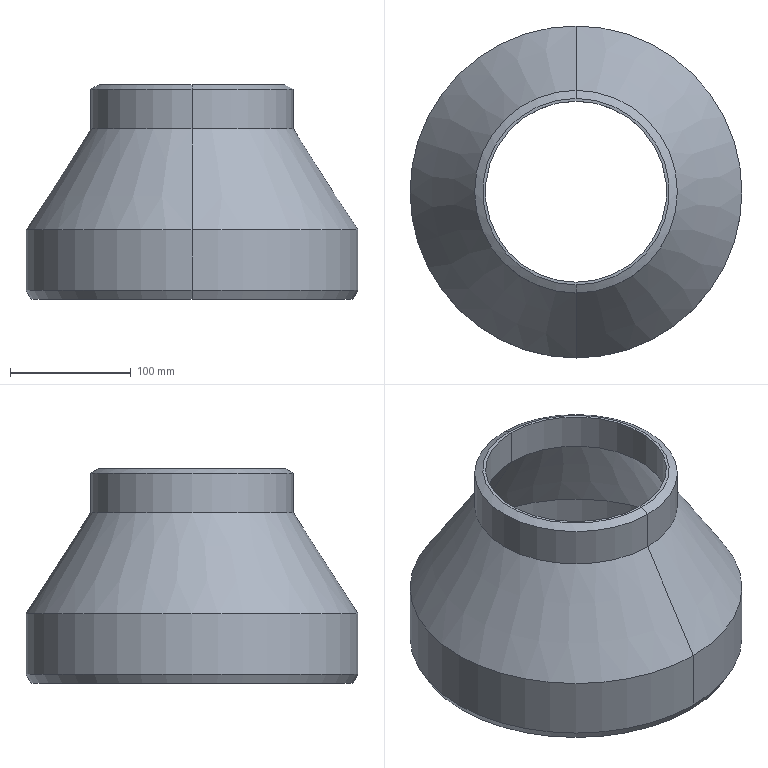Part | NX | features Resize Face 2, BREP 1 | 1 solid | 18 faces | box 275 x 275 x 178 mm | volume 1214659 mm3 | cone 8 | cylinder 8 | plane 2 | commonest cylinder face diameters 150 x2 168 x2 250 x2 275 x2
STEP:
#1=CARTESIAN_POINT('',(0.,-77.25,0.));
#2=VERTEX_POINT('',#1);
#3=CARTESIAN_POINT('',(0.,77.25,0.));
#4=VERTEX_POINT('',#3);
#5=CARTESIAN_POINT('',(0.,0.,0.));
#6=DIRECTION('',(0.,0.,1.));
#7=DIRECTION('',(0.,-1.,0.));
#8=AXIS2_PLACEMENT_3D('',#5,#6,#7);
#9=CIRCLE('',#8,77.25);
#10=EDGE_CURVE('',#2,#4,#9,.T.);
#11=ORIENTED_EDGE('',*,*,#10,.F.);
#12=CARTESIAN_POINT('',(0.,-84.,-3.897));
#13=VERTEX_POINT('',#12);
#14=CARTESIAN_POINT('',(0.,-79.5,-1.299));
#15=DIRECTION('',(0.,-0.866,-0.5));
#16=VECTOR('',#15,1000.);
#17=LINE('',#14,#16);
#18=EDGE_CURVE('',#2,#13,#17,.T.);
#19=ORIENTED_EDGE('',*,*,#18,.T.);
#20=CARTESIAN_POINT('',(0.,84.,-3.897));
#21=VERTEX_POINT('',#20);
#22=CARTESIAN_POINT('',(0.,0.,-3.897));
#23=DIRECTION('',(0.,0.,-1.));
#24=DIRECTION('',(0.,1.,0.));
#25=AXIS2_PLACEMENT_3D('',#22,#23,#24);
#26=CIRCLE('',#25,84.);
#27=EDGE_CURVE('',#21,#13,#26,.T.);
#28=ORIENTED_EDGE('',*,*,#27,.F.);
#29=CARTESIAN_POINT('',(0.,79.5,-1.299));
#30=DIRECTION('',(0.,0.866,-0.5));
#31=VECTOR('',#30,1000.);
#32=LINE('',#29,#31);
#33=EDGE_CURVE('',#4,#21,#32,.T.);
#34=ORIENTED_EDGE('',*,*,#33,.F.);
#35=EDGE_LOOP('',(#11,#19,#28,#34));
#36=FACE_BOUND('',#35,.T.);
#37=CARTESIAN_POINT('',(0.,0.,-1.299));
#38=DIRECTION('',(0.,0.,-1.));
#39=DIRECTION('',(0.,-1.,0.));
#40=AXIS2_PLACEMENT_3D('',#37,#38,#39);
#41=CONICAL_SURFACE('',#40,79.5,1.047);
#42=ADVANCED_FACE('',(#36),#41,.T.);
#43=CARTESIAN_POINT('',(0.,133.18,-178.));
#44=VERTEX_POINT('',#43);
#45=CARTESIAN_POINT('',(0.,-133.18,-178.));
#46=VERTEX_POINT('',#45);
#47=CARTESIAN_POINT('',(0.,0.,-178.));
#48=DIRECTION('',(0.,0.,-1.));
#49=DIRECTION('',(0.,1.,0.));
#50=AXIS2_PLACEMENT_3D('',#47,#48,#49);
#51=CIRCLE('',#50,133.18);
#52=EDGE_CURVE('',#44,#46,#51,.T.);
#53=ORIENTED_EDGE('',*,*,#52,.F.);
#54=CARTESIAN_POINT('',(0.,137.5,-170.518));
#55=VERTEX_POINT('',#54);
#56=CARTESIAN_POINT('',(0.,133.18,-178.));
#57=DIRECTION('',(0.,0.5,0.866));
#58=VECTOR('',#57,1000.);
#59=LINE('',#56,#58);
#60=EDGE_CURVE('',#55,#44,#59,.F.);
#61=ORIENTED_EDGE('',*,*,#60,.F.);
#62=CARTESIAN_POINT('',(0.,-137.5,-170.518));
#63=VERTEX_POINT('',#62);
#64=CARTESIAN_POINT('',(0.,0.,-170.518));
#65=DIRECTION('',(0.,0.,1.));
#66=DIRECTION('',(0.,-1.,0.));
#67=AXIS2_PLACEMENT_3D('',#64,#65,#66);
#68=CIRCLE('',#67,137.5);
#69=EDGE_CURVE('',#63,#55,#68,.T.);
#70=ORIENTED_EDGE('',*,*,#69,.F.);
#71=CARTESIAN_POINT('',(0.,-133.18,-178.));
#72=DIRECTION('',(0.,-0.5,0.866));
#73=VECTOR('',#72,1000.);
#74=LINE('',#71,#73);
#75=EDGE_CURVE('',#63,#46,#74,.F.);
#76=ORIENTED_EDGE('',*,*,#75,.T.);
#77=EDGE_LOOP('',(#53,#61,#70,#76));
#78=FACE_BOUND('',#77,.T.);
#79=CARTESIAN_POINT('',(0.,0.,-178.));
#80=DIRECTION('',(0.,0.,1.));
#81=DIRECTION('',(0.,1.,0.));
#82=AXIS2_PLACEMENT_3D('',#79,#80,#81);
#83=CONICAL_SURFACE('',#82,133.18,0.5236);
#84=ADVANCED_FACE('',(#78),#83,.T.);
#85=CARTESIAN_POINT('',(0.,-75.,0.));
#86=VERTEX_POINT('',#85);
#87=CARTESIAN_POINT('',(0.,75.,0.));
#88=VERTEX_POINT('',#87);
#89=CARTESIAN_POINT('',(0.,0.,0.));
#90=DIRECTION('',(0.,0.,-1.));
#91=DIRECTION('',(0.,1.,0.));
#92=AXIS2_PLACEMENT_3D('',#89,#90,#91);
#93=CIRCLE('',#92,75.);
#94=EDGE_CURVE('',#86,#88,#93,.T.);
#95=ORIENTED_EDGE('',*,*,#94,.F.);
#96=CARTESIAN_POINT('',(0.,-75.,-29.667));
#97=VERTEX_POINT('',#96);
#98=CARTESIAN_POINT('',(0.,-75.,-178.));
#99=DIRECTION('',(0.,0.,-1.));
#100=VECTOR('',#99,1000.);
#101=LINE('',#98,#100);
#102=EDGE_CURVE('',#86,#97,#101,.T.);
#103=ORIENTED_EDGE('',*,*,#102,.T.);
#104=CARTESIAN_POINT('',(0.,75.,-29.667));
#105=VERTEX_POINT('',#104);
#106=CARTESIAN_POINT('',(0.,0.,-29.667));
#107=DIRECTION('',(0.,0.,-1.));
#108=DIRECTION('',(0.,1.,0.));
#109=AXIS2_PLACEMENT_3D('',#106,#107,#108);
#110=CIRCLE('',#109,75.);
#111=EDGE_CURVE('',#97,#105,#110,.T.);
#112=ORIENTED_EDGE('',*,*,#111,.T.);
#113=CARTESIAN_POINT('',(0.,75.,-178.));
#114=DIRECTION('',(0.,0.,-1.));
#115=VECTOR('',#114,1000.);
#116=LINE('',#113,#115);
#117=EDGE_CURVE('',#88,#105,#116,.T.);
#118=ORIENTED_EDGE('',*,*,#117,.F.);
#119=EDGE_LOOP('',(#95,#103,#112,#118));
#120=FACE_BOUND('',#119,.T.);
#121=CARTESIAN_POINT('',(0.,0.,-178.));
#122=DIRECTION('',(0.,0.,-1.));
#123=DIRECTION('',(0.,-1.,0.));
#124=AXIS2_PLACEMENT_3D('',#121,#122,#123);
#125=CYLINDRICAL_SURFACE('',#124,75.);
#126=ADVANCED_FACE('',(#120),#125,.F.);
#127=ORIENTED_EDGE('',*,*,#111,.F.);
#128=CARTESIAN_POINT('',(0.,-125.,-118.667));
#129=VERTEX_POINT('',#128);
#130=CARTESIAN_POINT('',(0.,-75.,-29.667));
#131=DIRECTION('',(0.,-0.4898,-0.8718));
#132=VECTOR('',#131,1000.);
#133=LINE('',#130,#132);
#134=EDGE_CURVE('',#97,#129,#133,.T.);
#135=ORIENTED_EDGE('',*,*,#134,.T.);
#136=CARTESIAN_POINT('',(0.,125.,-118.667));
#137=VERTEX_POINT('',#136);
#138=CARTESIAN_POINT('',(0.,0.,-118.667));
#139=DIRECTION('',(0.,0.,-1.));
#140=DIRECTION('',(0.,1.,0.));
#141=AXIS2_PLACEMENT_3D('',#138,#139,#140);
#142=CIRCLE('',#141,125.);
#143=EDGE_CURVE('',#129,#137,#142,.T.);
#144=ORIENTED_EDGE('',*,*,#143,.T.);
#145=CARTESIAN_POINT('',(0.,75.,-29.667));
#146=DIRECTION('',(0.,0.4898,-0.8718));
#147=VECTOR('',#146,1000.);
#148=LINE('',#145,#147);
#149=EDGE_CURVE('',#105,#137,#148,.T.);
#150=ORIENTED_EDGE('',*,*,#149,.F.);
#151=EDGE_LOOP('',(#127,#135,#144,#150));
#152=FACE_BOUND('',#151,.T.);
#153=CARTESIAN_POINT('',(0.,0.,-29.667));
#154=DIRECTION('',(0.,0.,-1.));
#155=DIRECTION('',(0.,-1.,0.));
#156=AXIS2_PLACEMENT_3D('',#153,#154,#155);
#157=CONICAL_SURFACE('',#156,75.,0.5119);
#158=ADVANCED_FACE('',(#152),#157,.F.);
#159=ORIENTED_EDGE('',*,*,#143,.F.);
#160=CARTESIAN_POINT('',(0.,-125.,-178.));
#161=VERTEX_POINT('',#160);
#162=CARTESIAN_POINT('',(0.,-125.,-178.));
#163=DIRECTION('',(0.,0.,-1.));
#164=VECTOR('',#163,1000.);
#165=LINE('',#162,#164);
#166=EDGE_CURVE('',#129,#161,#165,.T.);
#167=ORIENTED_EDGE('',*,*,#166,.T.);
#168=CARTESIAN_POINT('',(0.,125.,-178.));
#169=VERTEX_POINT('',#168);
#170=CARTESIAN_POINT('',(0.,0.,-178.));
#171=DIRECTION('',(0.,0.,-1.));
#172=DIRECTION('',(0.,1.,0.));
#173=AXIS2_PLACEMENT_3D('',#170,#171,#172);
#174=CIRCLE('',#173,125.);
#175=EDGE_CURVE('',#161,#169,#174,.T.);
#176=ORIENTED_EDGE('',*,*,#175,.T.);
#177=CARTESIAN_POINT('',(0.,125.,-178.));
#178=DIRECTION('',(0.,0.,-1.));
#179=VECTOR('',#178,1000.);
#180=LINE('',#177,#179);
#181=EDGE_CURVE('',#137,#169,#180,.T.);
#182=ORIENTED_EDGE('',*,*,#181,.F.);
#183=EDGE_LOOP('',(#159,#167,#176,#182));
#184=FACE_BOUND('',#183,.T.);
#185=CARTESIAN_POINT('',(0.,0.,-178.));
#186=DIRECTION('',(0.,0.,-1.));
#187=DIRECTION('',(0.,-1.,0.));
#188=AXIS2_PLACEMENT_3D('',#185,#186,#187);
#189=CYLINDRICAL_SURFACE('',#188,125.);
#190=ADVANCED_FACE('',(#184),#189,.F.);
#191=CARTESIAN_POINT('',(0.,137.5,-120.228));
#192=VERTEX_POINT('',#191);
#193=CARTESIAN_POINT('',(0.,-137.5,-120.228));
#194=VERTEX_POINT('',#193);
#195=CARTESIAN_POINT('',(0.,0.,-120.228));
#196=DIRECTION('',(0.,0.,-1.));
#197=DIRECTION('',(0.,1.,0.));
#198=AXIS2_PLACEMENT_3D('',#195,#196,#197);
#199=CIRCLE('',#198,137.5);
#200=EDGE_CURVE('',#192,#194,#199,.T.);
#201=ORIENTED_EDGE('',*,*,#200,.T.);
#202=CARTESIAN_POINT('',(0.,-137.5,-178.));
#203=DIRECTION('',(0.,0.,-1.));
#204=VECTOR('',#203,1000.);
#205=LINE('',#202,#204);
#206=EDGE_CURVE('',#194,#63,#205,.T.);
#207=ORIENTED_EDGE('',*,*,#206,.T.);
#208=ORIENTED_EDGE('',*,*,#69,.T.);
#209=CARTESIAN_POINT('',(0.,137.5,-178.));
#210=DIRECTION('',(0.,0.,-1.));
#211=VECTOR('',#210,1000.);
#212=LINE('',#209,#211);
#213=EDGE_CURVE('',#192,#55,#212,.T.);
#214=ORIENTED_EDGE('',*,*,#213,.F.);
#215=EDGE_LOOP('',(#201,#207,#208,#214));
#216=FACE_BOUND('',#215,.T.);
#217=CARTESIAN_POINT('',(0.,0.,-178.));
#218=DIRECTION('',(0.,0.,-1.));
#219=DIRECTION('',(0.,-1.,0.));
#220=AXIS2_PLACEMENT_3D('',#217,#218,#219);
#221=CYLINDRICAL_SURFACE('',#220,137.5);
#222=ADVANCED_FACE('',(#216),#221,.T.);
#223=CARTESIAN_POINT('',(0.,84.,-36.693));
#224=VERTEX_POINT('',#223);
#225=CARTESIAN_POINT('',(0.,-84.,-36.693));
#226=VERTEX_POINT('',#225);
#227=CARTESIAN_POINT('',(0.,0.,-36.693));
#228=DIRECTION('',(0.,0.,-1.));
#229=DIRECTION('',(0.,1.,0.));
#230=AXIS2_PLACEMENT_3D('',#227,#228,#229);
#231=CIRCLE('',#230,84.);
#232=EDGE_CURVE('',#224,#226,#231,.T.);
#233=ORIENTED_EDGE('',*,*,#232,.T.);
#234=CARTESIAN_POINT('',(0.,-136.5,-118.667));
#235=DIRECTION('',(0.,-0.5393,-0.8421));
#236=VECTOR('',#235,1000.);
#237=LINE('',#234,#236);
#238=EDGE_CURVE('',#226,#194,#237,.T.);
#239=ORIENTED_EDGE('',*,*,#238,.T.);
#240=ORIENTED_EDGE('',*,*,#200,.F.);
#241=CARTESIAN_POINT('',(0.,136.5,-118.667));
#242=DIRECTION('',(0.,0.5393,-0.8421));
#243=VECTOR('',#242,1000.);
#244=LINE('',#241,#243);
#245=EDGE_CURVE('',#224,#192,#244,.T.);
#246=ORIENTED_EDGE('',*,*,#245,.F.);
#247=EDGE_LOOP('',(#233,#239,#240,#246));
#248=FACE_BOUND('',#247,.T.);
#249=CARTESIAN_POINT('',(0.,0.,-118.667));
#250=DIRECTION('',(0.,0.,-1.));
#251=DIRECTION('',(0.,-1.,0.));
#252=AXIS2_PLACEMENT_3D('',#249,#250,#251);
#253=CONICAL_SURFACE('',#252,136.5,0.5696);
#254=ADVANCED_FACE('',(#248),#253,.T.);
#255=ORIENTED_EDGE('',*,*,#27,.T.);
#256=CARTESIAN_POINT('',(0.,-84.,-178.));
#257=DIRECTION('',(0.,0.,-1.));
#258=VECTOR('',#257,1000.);
#259=LINE('',#256,#258);
#260=EDGE_CURVE('',#13,#226,#259,.T.);
#261=ORIENTED_EDGE('',*,*,#260,.T.);
#262=ORIENTED_EDGE('',*,*,#232,.F.);
#263=CARTESIAN_POINT('',(0.,84.,-178.));
#264=DIRECTION('',(0.,0.,-1.));
#265=VECTOR('',#264,1000.);
#266=LINE('',#263,#265);
#267=EDGE_CURVE('',#21,#224,#266,.T.);
#268=ORIENTED_EDGE('',*,*,#267,.F.);
#269=EDGE_LOOP('',(#255,#261,#262,#268));
#270=FACE_BOUND('',#269,.T.);
#271=CARTESIAN_POINT('',(0.,0.,-178.));
#272=DIRECTION('',(0.,0.,-1.));
#273=DIRECTION('',(0.,-1.,0.));
#274=AXIS2_PLACEMENT_3D('',#271,#272,#273);
#275=CYLINDRICAL_SURFACE('',#274,84.);
#276=ADVANCED_FACE('',(#270),#275,.T.);
#277=CARTESIAN_POINT('',(0.,0.,0.));
#278=DIRECTION('',(0.,0.,1.));
#279=DIRECTION('',(0.,-1.,0.));
#280=AXIS2_PLACEMENT_3D('',#277,#278,#279);
#281=CIRCLE('',#280,77.25);
#282=EDGE_CURVE('',#4,#2,#281,.T.);
#283=ORIENTED_EDGE('',*,*,#282,.T.);
#284=ORIENTED_EDGE('',*,*,#10,.T.);
#285=EDGE_LOOP('',(#283,#284));
#286=FACE_BOUND('',#285,.T.);
#287=CARTESIAN_POINT('',(0.,0.,0.));
#288=DIRECTION('',(0.,0.,-1.));
#289=DIRECTION('',(0.,1.,0.));
#290=AXIS2_PLACEMENT_3D('',#287,#288,#289);
#291=CIRCLE('',#290,75.);
#292=EDGE_CURVE('',#88,#86,#291,.T.);
#293=ORIENTED_EDGE('',*,*,#292,.T.);
#294=ORIENTED_EDGE('',*,*,#94,.T.);
#295=EDGE_LOOP('',(#293,#294));
#296=FACE_BOUND('',#295,.T.);
#297=CARTESIAN_POINT('',(0.,75.,0.));
#298=DIRECTION('',(0.,0.,1.));
#299=DIRECTION('',(0.,1.,0.));
#300=AXIS2_PLACEMENT_3D('',#297,#298,#299);
#301=PLANE('',#300);
#302=ADVANCED_FACE('',(#286,#296),#301,.T.);
#303=ORIENTED_EDGE('',*,*,#260,.F.);
#304=CARTESIAN_POINT('',(0.,0.,-3.897));
#305=DIRECTION('',(0.,0.,-1.));
#306=DIRECTION('',(0.,1.,0.));
#307=AXIS2_PLACEMENT_3D('',#304,#305,#306);
#308=CIRCLE('',#307,84.);
#309=EDGE_CURVE('',#13,#21,#308,.T.);
#310=ORIENTED_EDGE('',*,*,#309,.T.);
#311=ORIENTED_EDGE('',*,*,#267,.T.);
#312=CARTESIAN_POINT('',(0.,0.,-36.693));
#313=DIRECTION('',(0.,0.,-1.));
#314=DIRECTION('',(0.,1.,0.));
#315=AXIS2_PLACEMENT_3D('',#312,#313,#314);
#316=CIRCLE('',#315,84.);
#317=EDGE_CURVE('',#226,#224,#316,.T.);
#318=ORIENTED_EDGE('',*,*,#317,.F.);
#319=EDGE_LOOP('',(#303,#310,#311,#318));
#320=FACE_BOUND('',#319,.T.);
#321=CARTESIAN_POINT('',(0.,0.,-178.));
#322=DIRECTION('',(0.,0.,-1.));
#323=DIRECTION('',(0.,-1.,0.));
#324=AXIS2_PLACEMENT_3D('',#321,#322,#323);
#325=CYLINDRICAL_SURFACE('',#324,84.);
#326=ADVANCED_FACE('',(#320),#325,.T.);
#327=ORIENTED_EDGE('',*,*,#238,.F.);
#328=ORIENTED_EDGE('',*,*,#317,.T.);
#329=ORIENTED_EDGE('',*,*,#245,.T.);
#330=CARTESIAN_POINT('',(0.,0.,-120.228));
#331=DIRECTION('',(0.,0.,-1.));
#332=DIRECTION('',(0.,1.,0.));
#333=AXIS2_PLACEMENT_3D('',#330,#331,#332);
#334=CIRCLE('',#333,137.5);
#335=EDGE_CURVE('',#194,#192,#334,.T.);
#336=ORIENTED_EDGE('',*,*,#335,.F.);
#337=EDGE_LOOP('',(#327,#328,#329,#336));
#338=FACE_BOUND('',#337,.T.);
#339=CARTESIAN_POINT('',(0.,0.,-118.667));
#340=DIRECTION('',(0.,0.,-1.));
#341=DIRECTION('',(0.,-1.,0.));
#342=AXIS2_PLACEMENT_3D('',#339,#340,#341);
#343=CONICAL_SURFACE('',#342,136.5,0.5696);
#344=ADVANCED_FACE('',(#338),#343,.T.);
#345=ORIENTED_EDGE('',*,*,#206,.F.);
#346=ORIENTED_EDGE('',*,*,#335,.T.);
#347=ORIENTED_EDGE('',*,*,#213,.T.);
#348=CARTESIAN_POINT('',(0.,0.,-170.518));
#349=DIRECTION('',(0.,0.,1.));
#350=DIRECTION('',(0.,-1.,0.));
#351=AXIS2_PLACEMENT_3D('',#348,#349,#350);
#352=CIRCLE('',#351,137.5);
#353=EDGE_CURVE('',#55,#63,#352,.T.);
#354=ORIENTED_EDGE('',*,*,#353,.T.);
#355=EDGE_LOOP('',(#345,#346,#347,#354));
#356=FACE_BOUND('',#355,.T.);
#357=CARTESIAN_POINT('',(0.,0.,-178.));
#358=DIRECTION('',(0.,0.,-1.));
#359=DIRECTION('',(0.,-1.,0.));
#360=AXIS2_PLACEMENT_3D('',#357,#358,#359);
#361=CYLINDRICAL_SURFACE('',#360,137.5);
#362=ADVANCED_FACE('',(#356),#361,.T.);
#363=CARTESIAN_POINT('',(0.,0.,-178.));
#364=DIRECTION('',(0.,0.,-1.));
#365=DIRECTION('',(0.,1.,0.));
#366=AXIS2_PLACEMENT_3D('',#363,#364,#365);
#367=CIRCLE('',#366,133.18);
#368=EDGE_CURVE('',#46,#44,#367,.T.);
#369=ORIENTED_EDGE('',*,*,#368,.T.);
#370=ORIENTED_EDGE('',*,*,#52,.T.);
#371=EDGE_LOOP('',(#369,#370));
#372=FACE_BOUND('',#371,.T.);
#373=CARTESIAN_POINT('',(0.,0.,-178.));
#374=DIRECTION('',(0.,0.,-1.));
#375=DIRECTION('',(0.,1.,0.));
#376=AXIS2_PLACEMENT_3D('',#373,#374,#375);
#377=CIRCLE('',#376,125.);
#378=EDGE_CURVE('',#169,#161,#377,.T.);
#379=ORIENTED_EDGE('',*,*,#378,.F.);
#380=ORIENTED_EDGE('',*,*,#175,.F.);
#381=EDGE_LOOP('',(#379,#380));
#382=FACE_BOUND('',#381,.T.);
#383=CARTESIAN_POINT('',(0.,136.5,-178.));
#384=DIRECTION('',(0.,0.,-1.));
#385=DIRECTION('',(0.,-1.,0.));
#386=AXIS2_PLACEMENT_3D('',#383,#384,#385);
#387=PLANE('',#386);
#388=ADVANCED_FACE('',(#372,#382),#387,.T.);
#389=ORIENTED_EDGE('',*,*,#166,.F.);
#390=CARTESIAN_POINT('',(0.,0.,-118.667));
#391=DIRECTION('',(0.,0.,-1.));
#392=DIRECTION('',(0.,1.,0.));
#393=AXIS2_PLACEMENT_3D('',#390,#391,#392);
#394=CIRCLE('',#393,125.);
#395=EDGE_CURVE('',#137,#129,#394,.T.);
#396=ORIENTED_EDGE('',*,*,#395,.F.);
#397=ORIENTED_EDGE('',*,*,#181,.T.);
#398=ORIENTED_EDGE('',*,*,#378,.T.);
#399=EDGE_LOOP('',(#389,#396,#397,#398));
#400=FACE_BOUND('',#399,.T.);
#401=CARTESIAN_POINT('',(0.,0.,-178.));
#402=DIRECTION('',(0.,0.,-1.));
#403=DIRECTION('',(0.,-1.,0.));
#404=AXIS2_PLACEMENT_3D('',#401,#402,#403);
#405=CYLINDRICAL_SURFACE('',#404,125.);
#406=ADVANCED_FACE('',(#400),#405,.F.);
#407=ORIENTED_EDGE('',*,*,#134,.F.);
#408=CARTESIAN_POINT('',(0.,0.,-29.667));
#409=DIRECTION('',(0.,0.,-1.));
#410=DIRECTION('',(0.,1.,0.));
#411=AXIS2_PLACEMENT_3D('',#408,#409,#410);
#412=CIRCLE('',#411,75.);
#413=EDGE_CURVE('',#105,#97,#412,.T.);
#414=ORIENTED_EDGE('',*,*,#413,.F.);
#415=ORIENTED_EDGE('',*,*,#149,.T.);
#416=ORIENTED_EDGE('',*,*,#395,.T.);
#417=EDGE_LOOP('',(#407,#414,#415,#416));
#418=FACE_BOUND('',#417,.T.);
#419=CARTESIAN_POINT('',(0.,0.,-29.667));
#420=DIRECTION('',(0.,0.,-1.));
#421=DIRECTION('',(0.,-1.,0.));
#422=AXIS2_PLACEMENT_3D('',#419,#420,#421);
#423=CONICAL_SURFACE('',#422,75.,0.5119);
#424=ADVANCED_FACE('',(#418),#423,.F.);
#425=ORIENTED_EDGE('',*,*,#102,.F.);
#426=ORIENTED_EDGE('',*,*,#292,.F.);
#427=ORIENTED_EDGE('',*,*,#117,.T.);
#428=ORIENTED_EDGE('',*,*,#413,.T.);
#429=EDGE_LOOP('',(#425,#426,#427,#428));
#430=FACE_BOUND('',#429,.T.);
#431=CARTESIAN_POINT('',(0.,0.,-178.));
#432=DIRECTION('',(0.,0.,-1.));
#433=DIRECTION('',(0.,-1.,0.));
#434=AXIS2_PLACEMENT_3D('',#431,#432,#433);
#435=CYLINDRICAL_SURFACE('',#434,75.);
#436=ADVANCED_FACE('',(#430),#435,.F.);
#437=ORIENTED_EDGE('',*,*,#60,.T.);
#438=ORIENTED_EDGE('',*,*,#368,.F.);
#439=ORIENTED_EDGE('',*,*,#75,.F.);
#440=ORIENTED_EDGE('',*,*,#353,.F.);
#441=EDGE_LOOP('',(#437,#438,#439,#440));
#442=FACE_BOUND('',#441,.T.);
#443=CARTESIAN_POINT('',(0.,0.,-178.));
#444=DIRECTION('',(0.,0.,1.));
#445=DIRECTION('',(0.,1.,0.));
#446=AXIS2_PLACEMENT_3D('',#443,#444,#445);
#447=CONICAL_SURFACE('',#446,133.18,0.5236);
#448=ADVANCED_FACE('',(#442),#447,.T.);
#449=ORIENTED_EDGE('',*,*,#18,.F.);
#450=ORIENTED_EDGE('',*,*,#282,.F.);
#451=ORIENTED_EDGE('',*,*,#33,.T.);
#452=ORIENTED_EDGE('',*,*,#309,.F.);
#453=EDGE_LOOP('',(#449,#450,#451,#452));
#454=FACE_BOUND('',#453,.T.);
#455=CARTESIAN_POINT('',(0.,0.,-1.299));
#456=DIRECTION('',(0.,0.,-1.));
#457=DIRECTION('',(0.,-1.,0.));
#458=AXIS2_PLACEMENT_3D('',#455,#456,#457);
#459=CONICAL_SURFACE('',#458,79.5,1.047);
#460=ADVANCED_FACE('',(#454),#459,.T.);
#461=CLOSED_SHELL('',(#42,#84,#126,#158,#190,#222,#254,#276,#302,#326,#344,#362,#388,#406,#424,#436,#448,#460));
#462=MANIFOLD_SOLID_BREP('',#461);
#463=(LENGTH_UNIT()NAMED_UNIT(*)SI_UNIT(.MILLI.,.METRE.));
#464=UNCERTAINTY_MEASURE_WITH_UNIT(LENGTH_MEASURE(0.00001),#463,'','');
#465=(NAMED_UNIT(*)PLANE_ANGLE_UNIT()SI_UNIT($,.RADIAN.));
#466=(NAMED_UNIT(*)SI_UNIT($,.STERADIAN.)SOLID_ANGLE_UNIT());
#467=(GEOMETRIC_REPRESENTATION_CONTEXT(3)GLOBAL_UNCERTAINTY_ASSIGNED_CONTEXT((#464))GLOBAL_UNIT_ASSIGNED_CONTEXT((#463,#465,#466))REPRESENTATION_CONTEXT('',''));
#468=ADVANCED_BREP_SHAPE_REPRESENTATION('',(#462),#467);